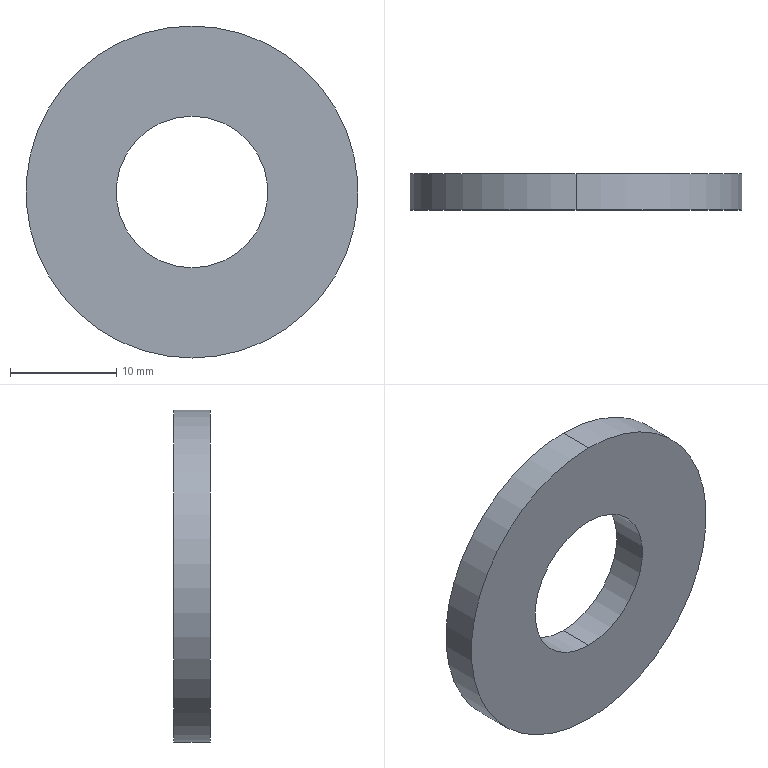Part | SolidWorks | features BaseBody 1 | 1 solid | 6 faces | box 31.3 x 3.4 x 31.3 mm | volume 2070 mm3 | cylinder 4 | plane 2 | commonest cylinder face diameters 14.3 x2 31.3 x2
STEP:
#1=CARTESIAN_POINT('',(624.451,114.75,24.933));
#2=VERTEX_POINT('',#1);
#3=CARTESIAN_POINT('',(624.451,114.75,10.633));
#4=VERTEX_POINT('',#3);
#5=CARTESIAN_POINT('',(624.451,114.75,17.783));
#6=DIRECTION('',(0.,1.,0.));
#7=DIRECTION('',(0.,0.,-1.));
#8=AXIS2_PLACEMENT_3D('',#5,#6,#7);
#9=CIRCLE('',#8,7.15);
#10=EDGE_CURVE('',#2,#4,#9,.T.);
#11=ORIENTED_EDGE('',*,*,#10,.F.);
#12=CARTESIAN_POINT('',(624.451,118.15,24.933));
#13=VERTEX_POINT('',#12);
#14=CARTESIAN_POINT('',(624.451,114.75,24.933));
#15=DIRECTION('',(0.,1.,0.));
#16=VECTOR('',#15,1000.);
#17=LINE('',#14,#16);
#18=EDGE_CURVE('',#2,#13,#17,.T.);
#19=ORIENTED_EDGE('',*,*,#18,.T.);
#20=CARTESIAN_POINT('',(624.451,118.15,10.633));
#21=VERTEX_POINT('',#20);
#22=CARTESIAN_POINT('',(624.451,118.15,17.783));
#23=DIRECTION('',(0.,1.,0.));
#24=DIRECTION('',(0.,0.,-1.));
#25=AXIS2_PLACEMENT_3D('',#22,#23,#24);
#26=CIRCLE('',#25,7.15);
#27=EDGE_CURVE('',#13,#21,#26,.T.);
#28=ORIENTED_EDGE('',*,*,#27,.T.);
#29=CARTESIAN_POINT('',(624.451,114.75,10.633));
#30=DIRECTION('',(0.,1.,0.));
#31=VECTOR('',#30,1000.);
#32=LINE('',#29,#31);
#33=EDGE_CURVE('',#4,#21,#32,.T.);
#34=ORIENTED_EDGE('',*,*,#33,.F.);
#35=EDGE_LOOP('',(#11,#19,#28,#34));
#36=FACE_OUTER_BOUND('',#35,.T.);
#37=CARTESIAN_POINT('',(624.451,114.75,17.783));
#38=DIRECTION('',(0.,1.,0.));
#39=DIRECTION('',(0.,0.,-1.));
#40=AXIS2_PLACEMENT_3D('',#37,#38,#39);
#41=CYLINDRICAL_SURFACE('',#40,7.15);
#42=ADVANCED_FACE('',(#36),#41,.F.);
#43=CARTESIAN_POINT('',(624.451,114.75,2.133));
#44=VERTEX_POINT('',#43);
#45=CARTESIAN_POINT('',(624.451,114.75,33.433));
#46=VERTEX_POINT('',#45);
#47=CARTESIAN_POINT('',(624.451,114.75,17.783));
#48=DIRECTION('',(0.,1.,0.));
#49=DIRECTION('',(0.,0.,-1.));
#50=AXIS2_PLACEMENT_3D('',#47,#48,#49);
#51=CIRCLE('',#50,15.65);
#52=EDGE_CURVE('',#44,#46,#51,.T.);
#53=ORIENTED_EDGE('',*,*,#52,.T.);
#54=CARTESIAN_POINT('',(624.451,118.15,33.433));
#55=VERTEX_POINT('',#54);
#56=CARTESIAN_POINT('',(624.451,114.75,33.433));
#57=DIRECTION('',(0.,1.,0.));
#58=VECTOR('',#57,1000.);
#59=LINE('',#56,#58);
#60=EDGE_CURVE('',#46,#55,#59,.T.);
#61=ORIENTED_EDGE('',*,*,#60,.T.);
#62=CARTESIAN_POINT('',(624.451,118.15,2.133));
#63=VERTEX_POINT('',#62);
#64=CARTESIAN_POINT('',(624.451,118.15,17.783));
#65=DIRECTION('',(0.,1.,0.));
#66=DIRECTION('',(0.,0.,-1.));
#67=AXIS2_PLACEMENT_3D('',#64,#65,#66);
#68=CIRCLE('',#67,15.65);
#69=EDGE_CURVE('',#63,#55,#68,.T.);
#70=ORIENTED_EDGE('',*,*,#69,.F.);
#71=CARTESIAN_POINT('',(624.451,114.75,2.133));
#72=DIRECTION('',(0.,1.,0.));
#73=VECTOR('',#72,1000.);
#74=LINE('',#71,#73);
#75=EDGE_CURVE('',#44,#63,#74,.T.);
#76=ORIENTED_EDGE('',*,*,#75,.F.);
#77=EDGE_LOOP('',(#53,#61,#70,#76));
#78=FACE_OUTER_BOUND('',#77,.T.);
#79=CARTESIAN_POINT('',(624.451,114.75,17.783));
#80=DIRECTION('',(0.,1.,0.));
#81=DIRECTION('',(0.,0.,-1.));
#82=AXIS2_PLACEMENT_3D('',#79,#80,#81);
#83=CYLINDRICAL_SURFACE('',#82,15.65);
#84=ADVANCED_FACE('',(#78),#83,.T.);
#85=CARTESIAN_POINT('',(624.451,118.15,17.783));
#86=DIRECTION('',(0.,1.,0.));
#87=DIRECTION('',(0.,0.,-1.));
#88=AXIS2_PLACEMENT_3D('',#85,#86,#87);
#89=CIRCLE('',#88,7.15);
#90=EDGE_CURVE('',#21,#13,#89,.T.);
#91=ORIENTED_EDGE('',*,*,#90,.F.);
#92=ORIENTED_EDGE('',*,*,#27,.F.);
#93=EDGE_LOOP('',(#91,#92));
#94=FACE_BOUND('',#93,.T.);
#95=ORIENTED_EDGE('',*,*,#69,.T.);
#96=CARTESIAN_POINT('',(624.451,118.15,17.783));
#97=DIRECTION('',(0.,1.,0.));
#98=DIRECTION('',(0.,0.,-1.));
#99=AXIS2_PLACEMENT_3D('',#96,#97,#98);
#100=CIRCLE('',#99,15.65);
#101=EDGE_CURVE('',#55,#63,#100,.T.);
#102=ORIENTED_EDGE('',*,*,#101,.T.);
#103=EDGE_LOOP('',(#95,#102));
#104=FACE_OUTER_BOUND('',#103,.T.);
#105=CARTESIAN_POINT('',(624.451,118.15,17.783));
#106=DIRECTION('',(0.,1.,0.));
#107=DIRECTION('',(1.,0.,0.));
#108=AXIS2_PLACEMENT_3D('',#105,#106,#107);
#109=PLANE('',#108);
#110=ADVANCED_FACE('',(#94,#104),#109,.T.);
#111=CARTESIAN_POINT('',(624.451,114.75,17.783));
#112=DIRECTION('',(0.,1.,0.));
#113=DIRECTION('',(0.,0.,-1.));
#114=AXIS2_PLACEMENT_3D('',#111,#112,#113);
#115=CIRCLE('',#114,7.15);
#116=EDGE_CURVE('',#4,#2,#115,.T.);
#117=ORIENTED_EDGE('',*,*,#116,.T.);
#118=ORIENTED_EDGE('',*,*,#10,.T.);
#119=EDGE_LOOP('',(#117,#118));
#120=FACE_BOUND('',#119,.T.);
#121=ORIENTED_EDGE('',*,*,#52,.F.);
#122=CARTESIAN_POINT('',(624.451,114.75,17.783));
#123=DIRECTION('',(0.,1.,0.));
#124=DIRECTION('',(0.,0.,-1.));
#125=AXIS2_PLACEMENT_3D('',#122,#123,#124);
#126=CIRCLE('',#125,15.65);
#127=EDGE_CURVE('',#46,#44,#126,.T.);
#128=ORIENTED_EDGE('',*,*,#127,.F.);
#129=EDGE_LOOP('',(#121,#128));
#130=FACE_OUTER_BOUND('',#129,.T.);
#131=CARTESIAN_POINT('',(624.451,114.75,17.783));
#132=DIRECTION('',(0.,1.,0.));
#133=DIRECTION('',(1.,0.,0.));
#134=AXIS2_PLACEMENT_3D('',#131,#132,#133);
#135=PLANE('',#134);
#136=ADVANCED_FACE('',(#120,#130),#135,.F.);
#137=ORIENTED_EDGE('',*,*,#60,.F.);
#138=ORIENTED_EDGE('',*,*,#127,.T.);
#139=ORIENTED_EDGE('',*,*,#75,.T.);
#140=ORIENTED_EDGE('',*,*,#101,.F.);
#141=EDGE_LOOP('',(#137,#138,#139,#140));
#142=FACE_OUTER_BOUND('',#141,.T.);
#143=CARTESIAN_POINT('',(624.451,114.75,17.783));
#144=DIRECTION('',(0.,1.,0.));
#145=DIRECTION('',(0.,0.,-1.));
#146=AXIS2_PLACEMENT_3D('',#143,#144,#145);
#147=CYLINDRICAL_SURFACE('',#146,15.65);
#148=ADVANCED_FACE('',(#142),#147,.T.);
#149=ORIENTED_EDGE('',*,*,#18,.F.);
#150=ORIENTED_EDGE('',*,*,#116,.F.);
#151=ORIENTED_EDGE('',*,*,#33,.T.);
#152=ORIENTED_EDGE('',*,*,#90,.T.);
#153=EDGE_LOOP('',(#149,#150,#151,#152));
#154=FACE_OUTER_BOUND('',#153,.T.);
#155=CARTESIAN_POINT('',(624.451,114.75,17.783));
#156=DIRECTION('',(0.,1.,0.));
#157=DIRECTION('',(0.,0.,-1.));
#158=AXIS2_PLACEMENT_3D('',#155,#156,#157);
#159=CYLINDRICAL_SURFACE('',#158,7.15);
#160=ADVANCED_FACE('',(#154),#159,.F.);
#161=CLOSED_SHELL('',(#42,#84,#110,#136,#148,#160));
#162=MANIFOLD_SOLID_BREP('',#161);
#163=CARTESIAN_POINT('',(0.,0.,0.));
#164=DIRECTION('',(0.,0.,1.));
#165=DIRECTION('',(1.,0.,0.));
#166=AXIS2_PLACEMENT_3D('',#163,#164,#165);
#167=(LENGTH_UNIT()NAMED_UNIT(*)SI_UNIT(.MILLI.,.METRE.));
#168=UNCERTAINTY_MEASURE_WITH_UNIT(LENGTH_MEASURE(0.00001),#167,'','');
#169=(NAMED_UNIT(*)PLANE_ANGLE_UNIT()SI_UNIT($,.RADIAN.));
#170=(NAMED_UNIT(*)SI_UNIT($,.STERADIAN.)SOLID_ANGLE_UNIT());
#171=(GEOMETRIC_REPRESENTATION_CONTEXT(3)GLOBAL_UNCERTAINTY_ASSIGNED_CONTEXT((#168))GLOBAL_UNIT_ASSIGNED_CONTEXT((#167,#169,#170))REPRESENTATION_CONTEXT('',''));
#172=ADVANCED_BREP_SHAPE_REPRESENTATION('',(#162,#166),#171);